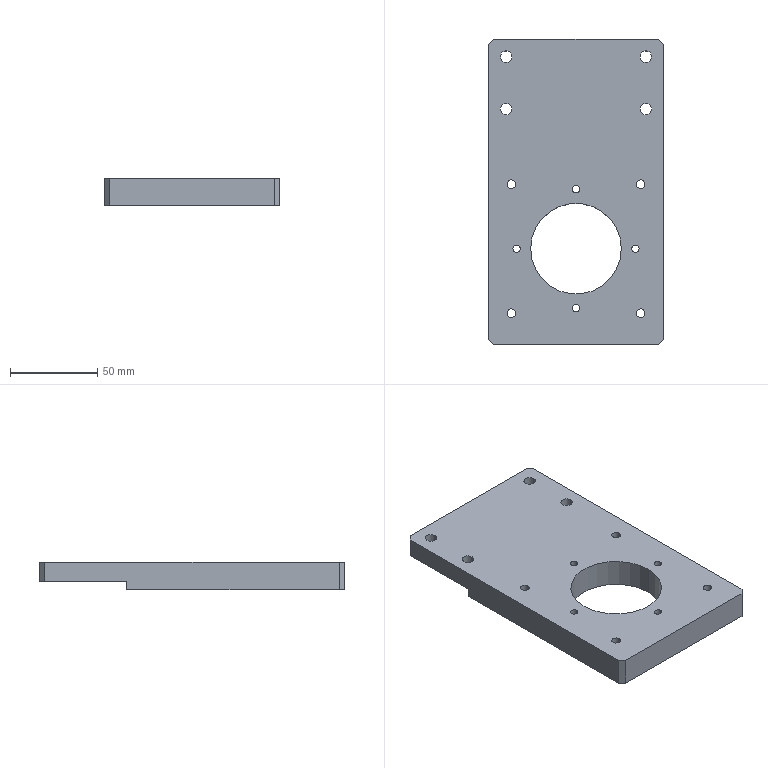Part | STEP file | MT-COMBO-119-S004 | 1 solid | 38 faces | box 100 x 175 x 16 mm | volume 217129 mm3 | cylinder 26 | plane 12 | commonest cylinder face diameters 4.2 x8 5 x8 6.6 x8 52 x2
STEP:
#1=CARTESIAN_POINT('',(36.1,-32.5,0.));
#2=VERTEX_POINT('',#1);
#3=CARTESIAN_POINT('',(31.9,-32.5,0.));
#4=VERTEX_POINT('',#3);
#5=CARTESIAN_POINT('',(34.,-32.5,0.));
#6=DIRECTION('',(0.,0.,-1.));
#7=DIRECTION('',(-1.,0.,0.));
#8=AXIS2_PLACEMENT_3D('',#5,#6,#7);
#9=CIRCLE('',#8,2.1);
#10=EDGE_CURVE('',#2,#4,#9,.T.);
#11=ORIENTED_EDGE('',*,*,#10,.F.);
#12=CARTESIAN_POINT('',(36.1,-32.5,-16.));
#13=VERTEX_POINT('',#12);
#14=CARTESIAN_POINT('',(36.1,-32.5,-16.));
#15=DIRECTION('',(0.,0.,-1.));
#16=VECTOR('',#15,1000.);
#17=LINE('',#14,#16);
#18=EDGE_CURVE('',#2,#13,#17,.T.);
#19=ORIENTED_EDGE('',*,*,#18,.T.);
#20=CARTESIAN_POINT('',(31.9,-32.5,-16.));
#21=VERTEX_POINT('',#20);
#22=CARTESIAN_POINT('',(34.,-32.5,-16.));
#23=DIRECTION('',(0.,0.,-1.));
#24=DIRECTION('',(-1.,0.,0.));
#25=AXIS2_PLACEMENT_3D('',#22,#23,#24);
#26=CIRCLE('',#25,2.1);
#27=EDGE_CURVE('',#13,#21,#26,.T.);
#28=ORIENTED_EDGE('',*,*,#27,.T.);
#29=CARTESIAN_POINT('',(31.9,-32.5,-16.));
#30=DIRECTION('',(0.,0.,-1.));
#31=VECTOR('',#30,1000.);
#32=LINE('',#29,#31);
#33=EDGE_CURVE('',#4,#21,#32,.T.);
#34=ORIENTED_EDGE('',*,*,#33,.F.);
#35=EDGE_LOOP('',(#11,#19,#28,#34));
#36=FACE_OUTER_BOUND('',#35,.T.);
#37=CARTESIAN_POINT('',(34.,-32.5,-16.));
#38=DIRECTION('',(0.,0.,-1.));
#39=DIRECTION('',(-1.,0.,0.));
#40=AXIS2_PLACEMENT_3D('',#37,#38,#39);
#41=CYLINDRICAL_SURFACE('',#40,2.1);
#42=ADVANCED_FACE('',(#36),#41,.F.);
#43=CARTESIAN_POINT('',(2.1,1.5,0.));
#44=VERTEX_POINT('',#43);
#45=CARTESIAN_POINT('',(-2.1,1.5,0.));
#46=VERTEX_POINT('',#45);
#47=CARTESIAN_POINT('',(0.,1.5,0.));
#48=DIRECTION('',(0.,0.,-1.));
#49=DIRECTION('',(-1.,0.,0.));
#50=AXIS2_PLACEMENT_3D('',#47,#48,#49);
#51=CIRCLE('',#50,2.1);
#52=EDGE_CURVE('',#44,#46,#51,.T.);
#53=ORIENTED_EDGE('',*,*,#52,.F.);
#54=CARTESIAN_POINT('',(2.1,1.5,-16.));
#55=VERTEX_POINT('',#54);
#56=CARTESIAN_POINT('',(2.1,1.5,-16.));
#57=DIRECTION('',(0.,0.,-1.));
#58=VECTOR('',#57,1000.);
#59=LINE('',#56,#58);
#60=EDGE_CURVE('',#44,#55,#59,.T.);
#61=ORIENTED_EDGE('',*,*,#60,.T.);
#62=CARTESIAN_POINT('',(-2.1,1.5,-16.));
#63=VERTEX_POINT('',#62);
#64=CARTESIAN_POINT('',(0.,1.5,-16.));
#65=DIRECTION('',(0.,0.,-1.));
#66=DIRECTION('',(-1.,0.,0.));
#67=AXIS2_PLACEMENT_3D('',#64,#65,#66);
#68=CIRCLE('',#67,2.1);
#69=EDGE_CURVE('',#55,#63,#68,.T.);
#70=ORIENTED_EDGE('',*,*,#69,.T.);
#71=CARTESIAN_POINT('',(-2.1,1.5,-16.));
#72=DIRECTION('',(0.,0.,-1.));
#73=VECTOR('',#72,1000.);
#74=LINE('',#71,#73);
#75=EDGE_CURVE('',#46,#63,#74,.T.);
#76=ORIENTED_EDGE('',*,*,#75,.F.);
#77=EDGE_LOOP('',(#53,#61,#70,#76));
#78=FACE_OUTER_BOUND('',#77,.T.);
#79=CARTESIAN_POINT('',(0.,1.5,-16.));
#80=DIRECTION('',(0.,0.,-1.));
#81=DIRECTION('',(-1.,0.,0.));
#82=AXIS2_PLACEMENT_3D('',#79,#80,#81);
#83=CYLINDRICAL_SURFACE('',#82,2.1);
#84=ADVANCED_FACE('',(#78),#83,.F.);
#85=CARTESIAN_POINT('',(2.1,-66.5,0.));
#86=VERTEX_POINT('',#85);
#87=CARTESIAN_POINT('',(-2.1,-66.5,0.));
#88=VERTEX_POINT('',#87);
#89=CARTESIAN_POINT('',(0.,-66.5,0.));
#90=DIRECTION('',(0.,0.,-1.));
#91=DIRECTION('',(-1.,0.,0.));
#92=AXIS2_PLACEMENT_3D('',#89,#90,#91);
#93=CIRCLE('',#92,2.1);
#94=EDGE_CURVE('',#86,#88,#93,.T.);
#95=ORIENTED_EDGE('',*,*,#94,.F.);
#96=CARTESIAN_POINT('',(2.1,-66.5,-16.));
#97=VERTEX_POINT('',#96);
#98=CARTESIAN_POINT('',(2.1,-66.5,-16.));
#99=DIRECTION('',(0.,0.,-1.));
#100=VECTOR('',#99,1000.);
#101=LINE('',#98,#100);
#102=EDGE_CURVE('',#86,#97,#101,.T.);
#103=ORIENTED_EDGE('',*,*,#102,.T.);
#104=CARTESIAN_POINT('',(-2.1,-66.5,-16.));
#105=VERTEX_POINT('',#104);
#106=CARTESIAN_POINT('',(0.,-66.5,-16.));
#107=DIRECTION('',(0.,0.,-1.));
#108=DIRECTION('',(-1.,0.,0.));
#109=AXIS2_PLACEMENT_3D('',#106,#107,#108);
#110=CIRCLE('',#109,2.1);
#111=EDGE_CURVE('',#97,#105,#110,.T.);
#112=ORIENTED_EDGE('',*,*,#111,.T.);
#113=CARTESIAN_POINT('',(-2.1,-66.5,-16.));
#114=DIRECTION('',(0.,0.,-1.));
#115=VECTOR('',#114,1000.);
#116=LINE('',#113,#115);
#117=EDGE_CURVE('',#88,#105,#116,.T.);
#118=ORIENTED_EDGE('',*,*,#117,.F.);
#119=EDGE_LOOP('',(#95,#103,#112,#118));
#120=FACE_OUTER_BOUND('',#119,.T.);
#121=CARTESIAN_POINT('',(0.,-66.5,-16.));
#122=DIRECTION('',(0.,0.,-1.));
#123=DIRECTION('',(-1.,0.,0.));
#124=AXIS2_PLACEMENT_3D('',#121,#122,#123);
#125=CYLINDRICAL_SURFACE('',#124,2.1);
#126=ADVANCED_FACE('',(#120),#125,.F.);
#127=CARTESIAN_POINT('',(-31.9,-32.5,0.));
#128=VERTEX_POINT('',#127);
#129=CARTESIAN_POINT('',(-36.1,-32.5,0.));
#130=VERTEX_POINT('',#129);
#131=CARTESIAN_POINT('',(-34.,-32.5,0.));
#132=DIRECTION('',(0.,0.,-1.));
#133=DIRECTION('',(-1.,0.,0.));
#134=AXIS2_PLACEMENT_3D('',#131,#132,#133);
#135=CIRCLE('',#134,2.1);
#136=EDGE_CURVE('',#128,#130,#135,.T.);
#137=ORIENTED_EDGE('',*,*,#136,.F.);
#138=CARTESIAN_POINT('',(-31.9,-32.5,-16.));
#139=VERTEX_POINT('',#138);
#140=CARTESIAN_POINT('',(-31.9,-32.5,-16.));
#141=DIRECTION('',(0.,0.,-1.));
#142=VECTOR('',#141,1000.);
#143=LINE('',#140,#142);
#144=EDGE_CURVE('',#128,#139,#143,.T.);
#145=ORIENTED_EDGE('',*,*,#144,.T.);
#146=CARTESIAN_POINT('',(-36.1,-32.5,-16.));
#147=VERTEX_POINT('',#146);
#148=CARTESIAN_POINT('',(-34.,-32.5,-16.));
#149=DIRECTION('',(0.,0.,-1.));
#150=DIRECTION('',(-1.,0.,0.));
#151=AXIS2_PLACEMENT_3D('',#148,#149,#150);
#152=CIRCLE('',#151,2.1);
#153=EDGE_CURVE('',#139,#147,#152,.T.);
#154=ORIENTED_EDGE('',*,*,#153,.T.);
#155=CARTESIAN_POINT('',(-36.1,-32.5,-16.));
#156=DIRECTION('',(0.,0.,-1.));
#157=VECTOR('',#156,1000.);
#158=LINE('',#155,#157);
#159=EDGE_CURVE('',#130,#147,#158,.T.);
#160=ORIENTED_EDGE('',*,*,#159,.F.);
#161=EDGE_LOOP('',(#137,#145,#154,#160));
#162=FACE_OUTER_BOUND('',#161,.T.);
#163=CARTESIAN_POINT('',(-34.,-32.5,-16.));
#164=DIRECTION('',(0.,0.,-1.));
#165=DIRECTION('',(-1.,0.,0.));
#166=AXIS2_PLACEMENT_3D('',#163,#164,#165);
#167=CYLINDRICAL_SURFACE('',#166,2.1);
#168=ADVANCED_FACE('',(#162),#167,.F.);
#169=CARTESIAN_POINT('',(-39.5,-69.5,-16.));
#170=VERTEX_POINT('',#169);
#171=CARTESIAN_POINT('',(-34.5,-69.5,-16.));
#172=VERTEX_POINT('',#171);
#173=CARTESIAN_POINT('',(-37.,-69.5,-16.));
#174=DIRECTION('',(0.,0.,-1.));
#175=DIRECTION('',(-1.,0.,0.));
#176=AXIS2_PLACEMENT_3D('',#173,#174,#175);
#177=CIRCLE('',#176,2.5);
#178=EDGE_CURVE('',#170,#172,#177,.T.);
#179=ORIENTED_EDGE('',*,*,#178,.T.);
#180=CARTESIAN_POINT('',(-34.5,-69.5,0.));
#181=VERTEX_POINT('',#180);
#182=CARTESIAN_POINT('',(-34.5,-69.5,0.));
#183=DIRECTION('',(0.,0.,1.));
#184=VECTOR('',#183,1000.);
#185=LINE('',#182,#184);
#186=EDGE_CURVE('',#172,#181,#185,.T.);
#187=ORIENTED_EDGE('',*,*,#186,.T.);
#188=CARTESIAN_POINT('',(-39.5,-69.5,0.));
#189=VERTEX_POINT('',#188);
#190=CARTESIAN_POINT('',(-37.,-69.5,0.));
#191=DIRECTION('',(0.,0.,-1.));
#192=DIRECTION('',(-1.,0.,0.));
#193=AXIS2_PLACEMENT_3D('',#190,#191,#192);
#194=CIRCLE('',#193,2.5);
#195=EDGE_CURVE('',#189,#181,#194,.T.);
#196=ORIENTED_EDGE('',*,*,#195,.F.);
#197=CARTESIAN_POINT('',(-39.5,-69.5,0.));
#198=DIRECTION('',(0.,0.,1.));
#199=VECTOR('',#198,1000.);
#200=LINE('',#197,#199);
#201=EDGE_CURVE('',#170,#189,#200,.T.);
#202=ORIENTED_EDGE('',*,*,#201,.F.);
#203=EDGE_LOOP('',(#179,#187,#196,#202));
#204=FACE_OUTER_BOUND('',#203,.T.);
#205=CARTESIAN_POINT('',(-37.,-69.5,0.));
#206=DIRECTION('',(0.,0.,1.));
#207=DIRECTION('',(-1.,0.,0.));
#208=AXIS2_PLACEMENT_3D('',#205,#206,#207);
#209=CYLINDRICAL_SURFACE('',#208,2.5);
#210=ADVANCED_FACE('',(#204),#209,.F.);
#211=CARTESIAN_POINT('',(34.5,-69.5,-16.));
#212=VERTEX_POINT('',#211);
#213=CARTESIAN_POINT('',(39.5,-69.5,-16.));
#214=VERTEX_POINT('',#213);
#215=CARTESIAN_POINT('',(37.,-69.5,-16.));
#216=DIRECTION('',(0.,0.,-1.));
#217=DIRECTION('',(-1.,0.,0.));
#218=AXIS2_PLACEMENT_3D('',#215,#216,#217);
#219=CIRCLE('',#218,2.5);
#220=EDGE_CURVE('',#212,#214,#219,.T.);
#221=ORIENTED_EDGE('',*,*,#220,.T.);
#222=CARTESIAN_POINT('',(39.5,-69.5,0.));
#223=VERTEX_POINT('',#222);
#224=CARTESIAN_POINT('',(39.5,-69.5,0.));
#225=DIRECTION('',(0.,0.,1.));
#226=VECTOR('',#225,1000.);
#227=LINE('',#224,#226);
#228=EDGE_CURVE('',#214,#223,#227,.T.);
#229=ORIENTED_EDGE('',*,*,#228,.T.);
#230=CARTESIAN_POINT('',(34.5,-69.5,0.));
#231=VERTEX_POINT('',#230);
#232=CARTESIAN_POINT('',(37.,-69.5,0.));
#233=DIRECTION('',(0.,0.,-1.));
#234=DIRECTION('',(-1.,0.,0.));
#235=AXIS2_PLACEMENT_3D('',#232,#233,#234);
#236=CIRCLE('',#235,2.5);
#237=EDGE_CURVE('',#231,#223,#236,.T.);
#238=ORIENTED_EDGE('',*,*,#237,.F.);
#239=CARTESIAN_POINT('',(34.5,-69.5,0.));
#240=DIRECTION('',(0.,0.,1.));
#241=VECTOR('',#240,1000.);
#242=LINE('',#239,#241);
#243=EDGE_CURVE('',#212,#231,#242,.T.);
#244=ORIENTED_EDGE('',*,*,#243,.F.);
#245=EDGE_LOOP('',(#221,#229,#238,#244));
#246=FACE_OUTER_BOUND('',#245,.T.);
#247=CARTESIAN_POINT('',(37.,-69.5,0.));
#248=DIRECTION('',(0.,0.,1.));
#249=DIRECTION('',(-1.,0.,0.));
#250=AXIS2_PLACEMENT_3D('',#247,#248,#249);
#251=CYLINDRICAL_SURFACE('',#250,2.5);
#252=ADVANCED_FACE('',(#246),#251,.F.);
#253=CARTESIAN_POINT('',(34.5,4.5,-16.));
#254=VERTEX_POINT('',#253);
#255=CARTESIAN_POINT('',(39.5,4.5,-16.));
#256=VERTEX_POINT('',#255);
#257=CARTESIAN_POINT('',(37.,4.5,-16.));
#258=DIRECTION('',(0.,0.,-1.));
#259=DIRECTION('',(-1.,0.,0.));
#260=AXIS2_PLACEMENT_3D('',#257,#258,#259);
#261=CIRCLE('',#260,2.5);
#262=EDGE_CURVE('',#254,#256,#261,.T.);
#263=ORIENTED_EDGE('',*,*,#262,.T.);
#264=CARTESIAN_POINT('',(39.5,4.5,0.));
#265=VERTEX_POINT('',#264);
#266=CARTESIAN_POINT('',(39.5,4.5,0.));
#267=DIRECTION('',(0.,0.,1.));
#268=VECTOR('',#267,1000.);
#269=LINE('',#266,#268);
#270=EDGE_CURVE('',#256,#265,#269,.T.);
#271=ORIENTED_EDGE('',*,*,#270,.T.);
#272=CARTESIAN_POINT('',(34.5,4.5,0.));
#273=VERTEX_POINT('',#272);
#274=CARTESIAN_POINT('',(37.,4.5,0.));
#275=DIRECTION('',(0.,0.,-1.));
#276=DIRECTION('',(-1.,0.,0.));
#277=AXIS2_PLACEMENT_3D('',#274,#275,#276);
#278=CIRCLE('',#277,2.5);
#279=EDGE_CURVE('',#273,#265,#278,.T.);
#280=ORIENTED_EDGE('',*,*,#279,.F.);
#281=CARTESIAN_POINT('',(34.5,4.5,0.));
#282=DIRECTION('',(0.,0.,1.));
#283=VECTOR('',#282,1000.);
#284=LINE('',#281,#283);
#285=EDGE_CURVE('',#254,#273,#284,.T.);
#286=ORIENTED_EDGE('',*,*,#285,.F.);
#287=EDGE_LOOP('',(#263,#271,#280,#286));
#288=FACE_OUTER_BOUND('',#287,.T.);
#289=CARTESIAN_POINT('',(37.,4.5,0.));
#290=DIRECTION('',(0.,0.,1.));
#291=DIRECTION('',(-1.,0.,0.));
#292=AXIS2_PLACEMENT_3D('',#289,#290,#291);
#293=CYLINDRICAL_SURFACE('',#292,2.5);
#294=ADVANCED_FACE('',(#288),#293,.F.);
#295=CARTESIAN_POINT('',(-39.5,4.5,-16.));
#296=VERTEX_POINT('',#295);
#297=CARTESIAN_POINT('',(-34.5,4.5,-16.));
#298=VERTEX_POINT('',#297);
#299=CARTESIAN_POINT('',(-37.,4.5,-16.));
#300=DIRECTION('',(0.,0.,-1.));
#301=DIRECTION('',(-1.,0.,0.));
#302=AXIS2_PLACEMENT_3D('',#299,#300,#301);
#303=CIRCLE('',#302,2.5);
#304=EDGE_CURVE('',#296,#298,#303,.T.);
#305=ORIENTED_EDGE('',*,*,#304,.T.);
#306=CARTESIAN_POINT('',(-34.5,4.5,0.));
#307=VERTEX_POINT('',#306);
#308=CARTESIAN_POINT('',(-34.5,4.5,0.));
#309=DIRECTION('',(0.,0.,1.));
#310=VECTOR('',#309,1000.);
#311=LINE('',#308,#310);
#312=EDGE_CURVE('',#298,#307,#311,.T.);
#313=ORIENTED_EDGE('',*,*,#312,.T.);
#314=CARTESIAN_POINT('',(-39.5,4.5,0.));
#315=VERTEX_POINT('',#314);
#316=CARTESIAN_POINT('',(-37.,4.5,0.));
#317=DIRECTION('',(0.,0.,-1.));
#318=DIRECTION('',(-1.,0.,0.));
#319=AXIS2_PLACEMENT_3D('',#316,#317,#318);
#320=CIRCLE('',#319,2.5);
#321=EDGE_CURVE('',#315,#307,#320,.T.);
#322=ORIENTED_EDGE('',*,*,#321,.F.);
#323=CARTESIAN_POINT('',(-39.5,4.5,0.));
#324=DIRECTION('',(0.,0.,1.));
#325=VECTOR('',#324,1000.);
#326=LINE('',#323,#325);
#327=EDGE_CURVE('',#296,#315,#326,.T.);
#328=ORIENTED_EDGE('',*,*,#327,.F.);
#329=EDGE_LOOP('',(#305,#313,#322,#328));
#330=FACE_OUTER_BOUND('',#329,.T.);
#331=CARTESIAN_POINT('',(-37.,4.5,0.));
#332=DIRECTION('',(0.,0.,1.));
#333=DIRECTION('',(-1.,0.,0.));
#334=AXIS2_PLACEMENT_3D('',#331,#332,#333);
#335=CYLINDRICAL_SURFACE('',#334,2.5);
#336=ADVANCED_FACE('',(#330),#335,.F.);
#337=CARTESIAN_POINT('',(-43.3,47.5,-11.));
#338=VERTEX_POINT('',#337);
#339=CARTESIAN_POINT('',(-36.7,47.5,-11.));
#340=VERTEX_POINT('',#339);
#341=CARTESIAN_POINT('',(-40.,47.5,-11.));
#342=DIRECTION('',(0.,0.,-1.));
#343=DIRECTION('',(-1.,0.,0.));
#344=AXIS2_PLACEMENT_3D('',#341,#342,#343);
#345=CIRCLE('',#344,3.3);
#346=EDGE_CURVE('',#338,#340,#345,.T.);
#347=ORIENTED_EDGE('',*,*,#346,.T.);
#348=CARTESIAN_POINT('',(-36.7,47.5,0.));
#349=VERTEX_POINT('',#348);
#350=CARTESIAN_POINT('',(-36.7,47.5,0.));
#351=DIRECTION('',(0.,0.,1.));
#352=VECTOR('',#351,1000.);
#353=LINE('',#350,#352);
#354=EDGE_CURVE('',#340,#349,#353,.T.);
#355=ORIENTED_EDGE('',*,*,#354,.T.);
#356=CARTESIAN_POINT('',(-43.3,47.5,0.));
#357=VERTEX_POINT('',#356);
#358=CARTESIAN_POINT('',(-40.,47.5,0.));
#359=DIRECTION('',(0.,0.,-1.));
#360=DIRECTION('',(-1.,0.,0.));
#361=AXIS2_PLACEMENT_3D('',#358,#359,#360);
#362=CIRCLE('',#361,3.3);
#363=EDGE_CURVE('',#357,#349,#362,.T.);
#364=ORIENTED_EDGE('',*,*,#363,.F.);
#365=CARTESIAN_POINT('',(-43.3,47.5,0.));
#366=DIRECTION('',(0.,0.,1.));
#367=VECTOR('',#366,1000.);
#368=LINE('',#365,#367);
#369=EDGE_CURVE('',#338,#357,#368,.T.);
#370=ORIENTED_EDGE('',*,*,#369,.F.);
#371=EDGE_LOOP('',(#347,#355,#364,#370));
#372=FACE_OUTER_BOUND('',#371,.T.);
#373=CARTESIAN_POINT('',(-40.,47.5,0.));
#374=DIRECTION('',(0.,0.,1.));
#375=DIRECTION('',(-1.,0.,0.));
#376=AXIS2_PLACEMENT_3D('',#373,#374,#375);
#377=CYLINDRICAL_SURFACE('',#376,3.3);
#378=ADVANCED_FACE('',(#372),#377,.F.);
#379=CARTESIAN_POINT('',(-43.3,77.5,-11.));
#380=VERTEX_POINT('',#379);
#381=CARTESIAN_POINT('',(-36.7,77.5,-11.));
#382=VERTEX_POINT('',#381);
#383=CARTESIAN_POINT('',(-40.,77.5,-11.));
#384=DIRECTION('',(0.,0.,-1.));
#385=DIRECTION('',(-1.,0.,0.));
#386=AXIS2_PLACEMENT_3D('',#383,#384,#385);
#387=CIRCLE('',#386,3.3);
#388=EDGE_CURVE('',#380,#382,#387,.T.);
#389=ORIENTED_EDGE('',*,*,#388,.T.);
#390=CARTESIAN_POINT('',(-36.7,77.5,0.));
#391=VERTEX_POINT('',#390);
#392=CARTESIAN_POINT('',(-36.7,77.5,0.));
#393=DIRECTION('',(0.,0.,1.));
#394=VECTOR('',#393,1000.);
#395=LINE('',#392,#394);
#396=EDGE_CURVE('',#382,#391,#395,.T.);
#397=ORIENTED_EDGE('',*,*,#396,.T.);
#398=CARTESIAN_POINT('',(-43.3,77.5,0.));
#399=VERTEX_POINT('',#398);
#400=CARTESIAN_POINT('',(-40.,77.5,0.));
#401=DIRECTION('',(0.,0.,-1.));
#402=DIRECTION('',(-1.,0.,0.));
#403=AXIS2_PLACEMENT_3D('',#400,#401,#402);
#404=CIRCLE('',#403,3.3);
#405=EDGE_CURVE('',#399,#391,#404,.T.);
#406=ORIENTED_EDGE('',*,*,#405,.F.);
#407=CARTESIAN_POINT('',(-43.3,77.5,0.));
#408=DIRECTION('',(0.,0.,1.));
#409=VECTOR('',#408,1000.);
#410=LINE('',#407,#409);
#411=EDGE_CURVE('',#380,#399,#410,.T.);
#412=ORIENTED_EDGE('',*,*,#411,.F.);
#413=EDGE_LOOP('',(#389,#397,#406,#412));
#414=FACE_OUTER_BOUND('',#413,.T.);
#415=CARTESIAN_POINT('',(-40.,77.5,0.));
#416=DIRECTION('',(0.,0.,1.));
#417=DIRECTION('',(-1.,0.,0.));
#418=AXIS2_PLACEMENT_3D('',#415,#416,#417);
#419=CYLINDRICAL_SURFACE('',#418,3.3);
#420=ADVANCED_FACE('',(#414),#419,.F.);
#421=CARTESIAN_POINT('',(36.7,77.5,-11.));
#422=VERTEX_POINT('',#421);
#423=CARTESIAN_POINT('',(43.3,77.5,-11.));
#424=VERTEX_POINT('',#423);
#425=CARTESIAN_POINT('',(40.,77.5,-11.));
#426=DIRECTION('',(0.,0.,-1.));
#427=DIRECTION('',(-1.,0.,0.));
#428=AXIS2_PLACEMENT_3D('',#425,#426,#427);
#429=CIRCLE('',#428,3.3);
#430=EDGE_CURVE('',#422,#424,#429,.T.);
#431=ORIENTED_EDGE('',*,*,#430,.T.);
#432=CARTESIAN_POINT('',(43.3,77.5,0.));
#433=VERTEX_POINT('',#432);
#434=CARTESIAN_POINT('',(43.3,77.5,0.));
#435=DIRECTION('',(0.,0.,1.));
#436=VECTOR('',#435,1000.);
#437=LINE('',#434,#436);
#438=EDGE_CURVE('',#424,#433,#437,.T.);
#439=ORIENTED_EDGE('',*,*,#438,.T.);
#440=CARTESIAN_POINT('',(36.7,77.5,0.));
#441=VERTEX_POINT('',#440);
#442=CARTESIAN_POINT('',(40.,77.5,0.));
#443=DIRECTION('',(0.,0.,-1.));
#444=DIRECTION('',(-1.,0.,0.));
#445=AXIS2_PLACEMENT_3D('',#442,#443,#444);
#446=CIRCLE('',#445,3.3);
#447=EDGE_CURVE('',#441,#433,#446,.T.);
#448=ORIENTED_EDGE('',*,*,#447,.F.);
#449=CARTESIAN_POINT('',(36.7,77.5,0.));
#450=DIRECTION('',(0.,0.,1.));
#451=VECTOR('',#450,1000.);
#452=LINE('',#449,#451);
#453=EDGE_CURVE('',#422,#441,#452,.T.);
#454=ORIENTED_EDGE('',*,*,#453,.F.);
#455=EDGE_LOOP('',(#431,#439,#448,#454));
#456=FACE_OUTER_BOUND('',#455,.T.);
#457=CARTESIAN_POINT('',(40.,77.5,0.));
#458=DIRECTION('',(0.,0.,1.));
#459=DIRECTION('',(-1.,0.,0.));
#460=AXIS2_PLACEMENT_3D('',#457,#458,#459);
#461=CYLINDRICAL_SURFACE('',#460,3.3);
#462=ADVANCED_FACE('',(#456),#461,.F.);
#463=CARTESIAN_POINT('',(36.7,47.5,-11.));
#464=VERTEX_POINT('',#463);
#465=CARTESIAN_POINT('',(43.3,47.5,-11.));
#466=VERTEX_POINT('',#465);
#467=CARTESIAN_POINT('',(40.,47.5,-11.));
#468=DIRECTION('',(0.,0.,-1.));
#469=DIRECTION('',(-1.,0.,0.));
#470=AXIS2_PLACEMENT_3D('',#467,#468,#469);
#471=CIRCLE('',#470,3.3);
#472=EDGE_CURVE('',#464,#466,#471,.T.);
#473=ORIENTED_EDGE('',*,*,#472,.T.);
#474=CARTESIAN_POINT('',(43.3,47.5,0.));
#475=VERTEX_POINT('',#474);
#476=CARTESIAN_POINT('',(43.3,47.5,0.));
#477=DIRECTION('',(0.,0.,1.));
#478=VECTOR('',#477,1000.);
#479=LINE('',#476,#478);
#480=EDGE_CURVE('',#466,#475,#479,.T.);
#481=ORIENTED_EDGE('',*,*,#480,.T.);
#482=CARTESIAN_POINT('',(36.7,47.5,0.));
#483=VERTEX_POINT('',#482);
#484=CARTESIAN_POINT('',(40.,47.5,0.));
#485=DIRECTION('',(0.,0.,-1.));
#486=DIRECTION('',(-1.,0.,0.));
#487=AXIS2_PLACEMENT_3D('',#484,#485,#486);
#488=CIRCLE('',#487,3.3);
#489=EDGE_CURVE('',#483,#475,#488,.T.);
#490=ORIENTED_EDGE('',*,*,#489,.F.);
#491=CARTESIAN_POINT('',(36.7,47.5,0.));
#492=DIRECTION('',(0.,0.,1.));
#493=VECTOR('',#492,1000.);
#494=LINE('',#491,#493);
#495=EDGE_CURVE('',#464,#483,#494,.T.);
#496=ORIENTED_EDGE('',*,*,#495,.F.);
#497=EDGE_LOOP('',(#473,#481,#490,#496));
#498=FACE_OUTER_BOUND('',#497,.T.);
#499=CARTESIAN_POINT('',(40.,47.5,0.));
#500=DIRECTION('',(0.,0.,1.));
#501=DIRECTION('',(-1.,0.,0.));
#502=AXIS2_PLACEMENT_3D('',#499,#500,#501);
#503=CYLINDRICAL_SURFACE('',#502,3.3);
#504=ADVANCED_FACE('',(#498),#503,.F.);
#505=CARTESIAN_POINT('',(-26.,-32.5,-16.));
#506=VERTEX_POINT('',#505);
#507=CARTESIAN_POINT('',(26.,-32.5,-16.));
#508=VERTEX_POINT('',#507);
#509=CARTESIAN_POINT('',(0.,-32.5,-16.));
#510=DIRECTION('',(0.,0.,-1.));
#511=DIRECTION('',(-1.,0.,0.));
#512=AXIS2_PLACEMENT_3D('',#509,#510,#511);
#513=CIRCLE('',#512,26.);
#514=EDGE_CURVE('',#506,#508,#513,.T.);
#515=ORIENTED_EDGE('',*,*,#514,.T.);
#516=CARTESIAN_POINT('',(26.,-32.5,0.));
#517=VERTEX_POINT('',#516);
#518=CARTESIAN_POINT('',(26.,-32.5,-16.));
#519=DIRECTION('',(0.,0.,1.));
#520=VECTOR('',#519,1000.);
#521=LINE('',#518,#520);
#522=EDGE_CURVE('',#508,#517,#521,.T.);
#523=ORIENTED_EDGE('',*,*,#522,.T.);
#524=CARTESIAN_POINT('',(-26.,-32.5,0.));
#525=VERTEX_POINT('',#524);
#526=CARTESIAN_POINT('',(0.,-32.5,0.));
#527=DIRECTION('',(0.,0.,-1.));
#528=DIRECTION('',(-1.,0.,0.));
#529=AXIS2_PLACEMENT_3D('',#526,#527,#528);
#530=CIRCLE('',#529,26.);
#531=EDGE_CURVE('',#525,#517,#530,.T.);
#532=ORIENTED_EDGE('',*,*,#531,.F.);
#533=CARTESIAN_POINT('',(-26.,-32.5,-16.));
#534=DIRECTION('',(0.,0.,1.));
#535=VECTOR('',#534,1000.);
#536=LINE('',#533,#535);
#537=EDGE_CURVE('',#506,#525,#536,.T.);
#538=ORIENTED_EDGE('',*,*,#537,.F.);
#539=EDGE_LOOP('',(#515,#523,#532,#538));
#540=FACE_OUTER_BOUND('',#539,.T.);
#541=CARTESIAN_POINT('',(0.,-32.5,-16.));
#542=DIRECTION('',(0.,0.,1.));
#543=DIRECTION('',(-1.,0.,0.));
#544=AXIS2_PLACEMENT_3D('',#541,#542,#543);
#545=CYLINDRICAL_SURFACE('',#544,26.);
#546=ADVANCED_FACE('',(#540),#545,.F.);
#547=CARTESIAN_POINT('',(50.,-84.5,-16.));
#548=VERTEX_POINT('',#547);
#549=CARTESIAN_POINT('',(50.,37.5,-16.));
#550=VERTEX_POINT('',#549);
#551=CARTESIAN_POINT('',(50.,-87.5,-16.));
#552=DIRECTION('',(0.,1.,0.));
#553=VECTOR('',#552,1000.);
#554=LINE('',#551,#553);
#555=EDGE_CURVE('',#548,#550,#554,.T.);
#556=ORIENTED_EDGE('',*,*,#555,.T.);
#557=CARTESIAN_POINT('',(50.,37.5,-11.));
#558=VERTEX_POINT('',#557);
#559=CARTESIAN_POINT('',(50.,37.5,-11.));
#560=DIRECTION('',(0.,0.,-1.));
#561=VECTOR('',#560,1000.);
#562=LINE('',#559,#561);
#563=EDGE_CURVE('',#558,#550,#562,.T.);
#564=ORIENTED_EDGE('',*,*,#563,.F.);
#565=CARTESIAN_POINT('',(50.,84.5,-11.));
#566=VERTEX_POINT('',#565);
#567=CARTESIAN_POINT('',(50.,87.5,-11.));
#568=DIRECTION('',(0.,1.,0.));
#569=VECTOR('',#568,1000.);
#570=LINE('',#567,#569);
#571=EDGE_CURVE('',#558,#566,#570,.T.);
#572=ORIENTED_EDGE('',*,*,#571,.T.);
#573=CARTESIAN_POINT('',(50.,84.5,0.));
#574=VERTEX_POINT('',#573);
#575=CARTESIAN_POINT('',(50.,84.5,-16.));
#576=DIRECTION('',(0.,0.,-1.));
#577=VECTOR('',#576,1000.);
#578=LINE('',#575,#577);
#579=EDGE_CURVE('',#574,#566,#578,.T.);
#580=ORIENTED_EDGE('',*,*,#579,.F.);
#581=CARTESIAN_POINT('',(50.,-84.5,0.));
#582=VERTEX_POINT('',#581);
#583=CARTESIAN_POINT('',(50.,-87.5,0.));
#584=DIRECTION('',(0.,1.,0.));
#585=VECTOR('',#584,1000.);
#586=LINE('',#583,#585);
#587=EDGE_CURVE('',#582,#574,#586,.T.);
#588=ORIENTED_EDGE('',*,*,#587,.F.);
#589=CARTESIAN_POINT('',(50.,-84.5,-16.));
#590=DIRECTION('',(0.,0.,1.));
#591=VECTOR('',#590,1000.);
#592=LINE('',#589,#591);
#593=EDGE_CURVE('',#548,#582,#592,.T.);
#594=ORIENTED_EDGE('',*,*,#593,.F.);
#595=EDGE_LOOP('',(#556,#564,#572,#580,#588,#594));
#596=FACE_OUTER_BOUND('',#595,.T.);
#597=CARTESIAN_POINT('',(50.,-87.5,-16.));
#598=DIRECTION('',(-1.,0.,0.));
#599=DIRECTION('',(0.,0.,-1.));
#600=AXIS2_PLACEMENT_3D('',#597,#598,#599);
#601=PLANE('',#600);
#602=ADVANCED_FACE('',(#596),#601,.F.);
#603=CARTESIAN_POINT('',(47.,87.5,0.));
#604=VERTEX_POINT('',#603);
#605=CARTESIAN_POINT('',(-47.,87.5,0.));
#606=VERTEX_POINT('',#605);
#607=CARTESIAN_POINT('',(-50.,87.5,0.));
#608=DIRECTION('',(-1.,0.,0.));
#609=VECTOR('',#608,1000.);
#610=LINE('',#607,#609);
#611=EDGE_CURVE('',#604,#606,#610,.T.);
#612=ORIENTED_EDGE('',*,*,#611,.F.);
#613=CARTESIAN_POINT('',(47.,87.5,-11.));
#614=VERTEX_POINT('',#613);
#615=CARTESIAN_POINT('',(47.,87.5,-16.));
#616=DIRECTION('',(0.,0.,1.));
#617=VECTOR('',#616,1000.);
#618=LINE('',#615,#617);
#619=EDGE_CURVE('',#614,#604,#618,.T.);
#620=ORIENTED_EDGE('',*,*,#619,.F.);
#621=CARTESIAN_POINT('',(-47.,87.5,-11.));
#622=VERTEX_POINT('',#621);
#623=CARTESIAN_POINT('',(50.,87.5,-11.));
#624=DIRECTION('',(-1.,0.,0.));
#625=VECTOR('',#624,1000.);
#626=LINE('',#623,#625);
#627=EDGE_CURVE('',#614,#622,#626,.T.);
#628=ORIENTED_EDGE('',*,*,#627,.T.);
#629=CARTESIAN_POINT('',(-47.,87.5,-16.));
#630=DIRECTION('',(0.,0.,-1.));
#631=VECTOR('',#630,1000.);
#632=LINE('',#629,#631);
#633=EDGE_CURVE('',#606,#622,#632,.T.);
#634=ORIENTED_EDGE('',*,*,#633,.F.);
#635=EDGE_LOOP('',(#612,#620,#628,#634));
#636=FACE_OUTER_BOUND('',#635,.T.);
#637=CARTESIAN_POINT('',(-50.,87.5,-16.));
#638=DIRECTION('',(0.,-1.,0.));
#639=DIRECTION('',(0.,0.,1.));
#640=AXIS2_PLACEMENT_3D('',#637,#638,#639);
#641=PLANE('',#640);
#642=ADVANCED_FACE('',(#636),#641,.F.);
#643=CARTESIAN_POINT('',(-50.,84.5,0.));
#644=VERTEX_POINT('',#643);
#645=CARTESIAN_POINT('',(-50.,-84.5,0.));
#646=VERTEX_POINT('',#645);
#647=CARTESIAN_POINT('',(-50.,-87.5,0.));
#648=DIRECTION('',(0.,-1.,0.));
#649=VECTOR('',#648,1000.);
#650=LINE('',#647,#649);
#651=EDGE_CURVE('',#644,#646,#650,.T.);
#652=ORIENTED_EDGE('',*,*,#651,.F.);
#653=CARTESIAN_POINT('',(-50.,84.5,-11.));
#654=VERTEX_POINT('',#653);
#655=CARTESIAN_POINT('',(-50.,84.5,-16.));
#656=DIRECTION('',(0.,0.,1.));
#657=VECTOR('',#656,1000.);
#658=LINE('',#655,#657);
#659=EDGE_CURVE('',#654,#644,#658,.T.);
#660=ORIENTED_EDGE('',*,*,#659,.F.);
#661=CARTESIAN_POINT('',(-50.,37.5,-11.));
#662=VERTEX_POINT('',#661);
#663=CARTESIAN_POINT('',(-50.,87.5,-11.));
#664=DIRECTION('',(0.,-1.,0.));
#665=VECTOR('',#664,1000.);
#666=LINE('',#663,#665);
#667=EDGE_CURVE('',#654,#662,#666,.T.);
#668=ORIENTED_EDGE('',*,*,#667,.T.);
#669=CARTESIAN_POINT('',(-50.,37.5,-16.));
#670=VERTEX_POINT('',#669);
#671=CARTESIAN_POINT('',(-50.,37.5,-11.));
#672=DIRECTION('',(0.,0.,-1.));
#673=VECTOR('',#672,1000.);
#674=LINE('',#671,#673);
#675=EDGE_CURVE('',#662,#670,#674,.T.);
#676=ORIENTED_EDGE('',*,*,#675,.T.);
#677=CARTESIAN_POINT('',(-50.,-84.5,-16.));
#678=VERTEX_POINT('',#677);
#679=CARTESIAN_POINT('',(-50.,-87.5,-16.));
#680=DIRECTION('',(0.,-1.,0.));
#681=VECTOR('',#680,1000.);
#682=LINE('',#679,#681);
#683=EDGE_CURVE('',#670,#678,#682,.T.);
#684=ORIENTED_EDGE('',*,*,#683,.T.);
#685=CARTESIAN_POINT('',(-50.,-84.5,-16.));
#686=DIRECTION('',(0.,0.,-1.));
#687=VECTOR('',#686,1000.);
#688=LINE('',#685,#687);
#689=EDGE_CURVE('',#646,#678,#688,.T.);
#690=ORIENTED_EDGE('',*,*,#689,.F.);
#691=EDGE_LOOP('',(#652,#660,#668,#676,#684,#690));
#692=FACE_OUTER_BOUND('',#691,.T.);
#693=CARTESIAN_POINT('',(-50.,-87.5,-16.));
#694=DIRECTION('',(1.,0.,0.));
#695=DIRECTION('',(0.,0.,1.));
#696=AXIS2_PLACEMENT_3D('',#693,#694,#695);
#697=PLANE('',#696);
#698=ADVANCED_FACE('',(#692),#697,.F.);
#699=CARTESIAN_POINT('',(-47.,-87.5,-16.));
#700=VERTEX_POINT('',#699);
#701=CARTESIAN_POINT('',(47.,-87.5,-16.));
#702=VERTEX_POINT('',#701);
#703=CARTESIAN_POINT('',(-50.,-87.5,-16.));
#704=DIRECTION('',(1.,0.,0.));
#705=VECTOR('',#704,1000.);
#706=LINE('',#703,#705);
#707=EDGE_CURVE('',#700,#702,#706,.T.);
#708=ORIENTED_EDGE('',*,*,#707,.T.);
#709=CARTESIAN_POINT('',(47.,-87.5,0.));
#710=VERTEX_POINT('',#709);
#711=CARTESIAN_POINT('',(47.,-87.5,-16.));
#712=DIRECTION('',(0.,0.,-1.));
#713=VECTOR('',#712,1000.);
#714=LINE('',#711,#713);
#715=EDGE_CURVE('',#710,#702,#714,.T.);
#716=ORIENTED_EDGE('',*,*,#715,.F.);
#717=CARTESIAN_POINT('',(-47.,-87.5,0.));
#718=VERTEX_POINT('',#717);
#719=CARTESIAN_POINT('',(-50.,-87.5,0.));
#720=DIRECTION('',(1.,0.,0.));
#721=VECTOR('',#720,1000.);
#722=LINE('',#719,#721);
#723=EDGE_CURVE('',#718,#710,#722,.T.);
#724=ORIENTED_EDGE('',*,*,#723,.F.);
#725=CARTESIAN_POINT('',(-47.,-87.5,-16.));
#726=DIRECTION('',(0.,0.,1.));
#727=VECTOR('',#726,1000.);
#728=LINE('',#725,#727);
#729=EDGE_CURVE('',#700,#718,#728,.T.);
#730=ORIENTED_EDGE('',*,*,#729,.F.);
#731=EDGE_LOOP('',(#708,#716,#724,#730));
#732=FACE_OUTER_BOUND('',#731,.T.);
#733=CARTESIAN_POINT('',(-50.,-87.5,-16.));
#734=DIRECTION('',(0.,1.,0.));
#735=DIRECTION('',(0.,0.,-1.));
#736=AXIS2_PLACEMENT_3D('',#733,#734,#735);
#737=PLANE('',#736);
#738=ADVANCED_FACE('',(#732),#737,.F.);
#739=CARTESIAN_POINT('',(34.,-32.5,-16.));
#740=DIRECTION('',(0.,0.,-1.));
#741=DIRECTION('',(-1.,0.,0.));
#742=AXIS2_PLACEMENT_3D('',#739,#740,#741);
#743=CIRCLE('',#742,2.1);
#744=EDGE_CURVE('',#21,#13,#743,.T.);
#745=ORIENTED_EDGE('',*,*,#744,.F.);
#746=ORIENTED_EDGE('',*,*,#27,.F.);
#747=EDGE_LOOP('',(#745,#746));
#748=FACE_BOUND('',#747,.T.);
#749=CARTESIAN_POINT('',(0.,1.5,-16.));
#750=DIRECTION('',(0.,0.,-1.));
#751=DIRECTION('',(-1.,0.,0.));
#752=AXIS2_PLACEMENT_3D('',#749,#750,#751);
#753=CIRCLE('',#752,2.1);
#754=EDGE_CURVE('',#63,#55,#753,.T.);
#755=ORIENTED_EDGE('',*,*,#754,.F.);
#756=ORIENTED_EDGE('',*,*,#69,.F.);
#757=EDGE_LOOP('',(#755,#756));
#758=FACE_BOUND('',#757,.T.);
#759=CARTESIAN_POINT('',(0.,-66.5,-16.));
#760=DIRECTION('',(0.,0.,-1.));
#761=DIRECTION('',(-1.,0.,0.));
#762=AXIS2_PLACEMENT_3D('',#759,#760,#761);
#763=CIRCLE('',#762,2.1);
#764=EDGE_CURVE('',#105,#97,#763,.T.);
#765=ORIENTED_EDGE('',*,*,#764,.F.);
#766=ORIENTED_EDGE('',*,*,#111,.F.);
#767=EDGE_LOOP('',(#765,#766));
#768=FACE_BOUND('',#767,.T.);
#769=CARTESIAN_POINT('',(-34.,-32.5,-16.));
#770=DIRECTION('',(0.,0.,-1.));
#771=DIRECTION('',(-1.,0.,0.));
#772=AXIS2_PLACEMENT_3D('',#769,#770,#771);
#773=CIRCLE('',#772,2.1);
#774=EDGE_CURVE('',#147,#139,#773,.T.);
#775=ORIENTED_EDGE('',*,*,#774,.F.);
#776=ORIENTED_EDGE('',*,*,#153,.F.);
#777=EDGE_LOOP('',(#775,#776));
#778=FACE_BOUND('',#777,.T.);
#779=ORIENTED_EDGE('',*,*,#178,.F.);
#780=CARTESIAN_POINT('',(-37.,-69.5,-16.));
#781=DIRECTION('',(0.,0.,-1.));
#782=DIRECTION('',(-1.,0.,0.));
#783=AXIS2_PLACEMENT_3D('',#780,#781,#782);
#784=CIRCLE('',#783,2.5);
#785=EDGE_CURVE('',#172,#170,#784,.T.);
#786=ORIENTED_EDGE('',*,*,#785,.F.);
#787=EDGE_LOOP('',(#779,#786));
#788=FACE_BOUND('',#787,.T.);
#789=ORIENTED_EDGE('',*,*,#220,.F.);
#790=CARTESIAN_POINT('',(37.,-69.5,-16.));
#791=DIRECTION('',(0.,0.,-1.));
#792=DIRECTION('',(-1.,0.,0.));
#793=AXIS2_PLACEMENT_3D('',#790,#791,#792);
#794=CIRCLE('',#793,2.5);
#795=EDGE_CURVE('',#214,#212,#794,.T.);
#796=ORIENTED_EDGE('',*,*,#795,.F.);
#797=EDGE_LOOP('',(#789,#796));
#798=FACE_BOUND('',#797,.T.);
#799=ORIENTED_EDGE('',*,*,#262,.F.);
#800=CARTESIAN_POINT('',(37.,4.5,-16.));
#801=DIRECTION('',(0.,0.,-1.));
#802=DIRECTION('',(-1.,0.,0.));
#803=AXIS2_PLACEMENT_3D('',#800,#801,#802);
#804=CIRCLE('',#803,2.5);
#805=EDGE_CURVE('',#256,#254,#804,.T.);
#806=ORIENTED_EDGE('',*,*,#805,.F.);
#807=EDGE_LOOP('',(#799,#806));
#808=FACE_BOUND('',#807,.T.);
#809=ORIENTED_EDGE('',*,*,#304,.F.);
#810=CARTESIAN_POINT('',(-37.,4.5,-16.));
#811=DIRECTION('',(0.,0.,-1.));
#812=DIRECTION('',(-1.,0.,0.));
#813=AXIS2_PLACEMENT_3D('',#810,#811,#812);
#814=CIRCLE('',#813,2.5);
#815=EDGE_CURVE('',#298,#296,#814,.T.);
#816=ORIENTED_EDGE('',*,*,#815,.F.);
#817=EDGE_LOOP('',(#809,#816));
#818=FACE_BOUND('',#817,.T.);
#819=ORIENTED_EDGE('',*,*,#514,.F.);
#820=CARTESIAN_POINT('',(0.,-32.5,-16.));
#821=DIRECTION('',(0.,0.,-1.));
#822=DIRECTION('',(-1.,0.,0.));
#823=AXIS2_PLACEMENT_3D('',#820,#821,#822);
#824=CIRCLE('',#823,26.);
#825=EDGE_CURVE('',#508,#506,#824,.T.);
#826=ORIENTED_EDGE('',*,*,#825,.F.);
#827=EDGE_LOOP('',(#819,#826));
#828=FACE_BOUND('',#827,.T.);
#829=ORIENTED_EDGE('',*,*,#683,.F.);
#830=CARTESIAN_POINT('',(50.,37.5,-16.));
#831=DIRECTION('',(1.,0.,0.));
#832=VECTOR('',#831,1000.);
#833=LINE('',#830,#832);
#834=EDGE_CURVE('',#670,#550,#833,.T.);
#835=ORIENTED_EDGE('',*,*,#834,.T.);
#836=ORIENTED_EDGE('',*,*,#555,.F.);
#837=CARTESIAN_POINT('',(50.,-84.5,-16.));
#838=DIRECTION('',(0.7071,0.7071,0.));
#839=VECTOR('',#838,1000.);
#840=LINE('',#837,#839);
#841=EDGE_CURVE('',#702,#548,#840,.T.);
#842=ORIENTED_EDGE('',*,*,#841,.F.);
#843=ORIENTED_EDGE('',*,*,#707,.F.);
#844=CARTESIAN_POINT('',(-47.,-87.5,-16.));
#845=DIRECTION('',(0.7071,-0.7071,0.));
#846=VECTOR('',#845,1000.);
#847=LINE('',#844,#846);
#848=EDGE_CURVE('',#678,#700,#847,.T.);
#849=ORIENTED_EDGE('',*,*,#848,.F.);
#850=EDGE_LOOP('',(#829,#835,#836,#842,#843,#849));
#851=FACE_OUTER_BOUND('',#850,.T.);
#852=CARTESIAN_POINT('',(0.,0.,-16.));
#853=DIRECTION('',(0.,0.,1.));
#854=DIRECTION('',(-1.,0.,0.));
#855=AXIS2_PLACEMENT_3D('',#852,#853,#854);
#856=PLANE('',#855);
#857=ADVANCED_FACE('',(#748,#758,#768,#778,#788,#798,#808,#818,#828,#851),#856,.F.);
#858=CARTESIAN_POINT('',(34.,-32.5,0.));
#859=DIRECTION('',(0.,0.,-1.));
#860=DIRECTION('',(-1.,0.,0.));
#861=AXIS2_PLACEMENT_3D('',#858,#859,#860);
#862=CIRCLE('',#861,2.1);
#863=EDGE_CURVE('',#4,#2,#862,.T.);
#864=ORIENTED_EDGE('',*,*,#863,.T.);
#865=ORIENTED_EDGE('',*,*,#10,.T.);
#866=EDGE_LOOP('',(#864,#865));
#867=FACE_BOUND('',#866,.T.);
#868=CARTESIAN_POINT('',(0.,1.5,0.));
#869=DIRECTION('',(0.,0.,-1.));
#870=DIRECTION('',(-1.,0.,0.));
#871=AXIS2_PLACEMENT_3D('',#868,#869,#870);
#872=CIRCLE('',#871,2.1);
#873=EDGE_CURVE('',#46,#44,#872,.T.);
#874=ORIENTED_EDGE('',*,*,#873,.T.);
#875=ORIENTED_EDGE('',*,*,#52,.T.);
#876=EDGE_LOOP('',(#874,#875));
#877=FACE_BOUND('',#876,.T.);
#878=CARTESIAN_POINT('',(0.,-66.5,0.));
#879=DIRECTION('',(0.,0.,-1.));
#880=DIRECTION('',(-1.,0.,0.));
#881=AXIS2_PLACEMENT_3D('',#878,#879,#880);
#882=CIRCLE('',#881,2.1);
#883=EDGE_CURVE('',#88,#86,#882,.T.);
#884=ORIENTED_EDGE('',*,*,#883,.T.);
#885=ORIENTED_EDGE('',*,*,#94,.T.);
#886=EDGE_LOOP('',(#884,#885));
#887=FACE_BOUND('',#886,.T.);
#888=CARTESIAN_POINT('',(-34.,-32.5,0.));
#889=DIRECTION('',(0.,0.,-1.));
#890=DIRECTION('',(-1.,0.,0.));
#891=AXIS2_PLACEMENT_3D('',#888,#889,#890);
#892=CIRCLE('',#891,2.1);
#893=EDGE_CURVE('',#130,#128,#892,.T.);
#894=ORIENTED_EDGE('',*,*,#893,.T.);
#895=ORIENTED_EDGE('',*,*,#136,.T.);
#896=EDGE_LOOP('',(#894,#895));
#897=FACE_BOUND('',#896,.T.);
#898=ORIENTED_EDGE('',*,*,#195,.T.);
#899=CARTESIAN_POINT('',(-37.,-69.5,0.));
#900=DIRECTION('',(0.,0.,-1.));
#901=DIRECTION('',(-1.,0.,0.));
#902=AXIS2_PLACEMENT_3D('',#899,#900,#901);
#903=CIRCLE('',#902,2.5);
#904=EDGE_CURVE('',#181,#189,#903,.T.);
#905=ORIENTED_EDGE('',*,*,#904,.T.);
#906=EDGE_LOOP('',(#898,#905));
#907=FACE_BOUND('',#906,.T.);
#908=ORIENTED_EDGE('',*,*,#237,.T.);
#909=CARTESIAN_POINT('',(37.,-69.5,0.));
#910=DIRECTION('',(0.,0.,-1.));
#911=DIRECTION('',(-1.,0.,0.));
#912=AXIS2_PLACEMENT_3D('',#909,#910,#911);
#913=CIRCLE('',#912,2.5);
#914=EDGE_CURVE('',#223,#231,#913,.T.);
#915=ORIENTED_EDGE('',*,*,#914,.T.);
#916=EDGE_LOOP('',(#908,#915));
#917=FACE_BOUND('',#916,.T.);
#918=ORIENTED_EDGE('',*,*,#279,.T.);
#919=CARTESIAN_POINT('',(37.,4.5,0.));
#920=DIRECTION('',(0.,0.,-1.));
#921=DIRECTION('',(-1.,0.,0.));
#922=AXIS2_PLACEMENT_3D('',#919,#920,#921);
#923=CIRCLE('',#922,2.5);
#924=EDGE_CURVE('',#265,#273,#923,.T.);
#925=ORIENTED_EDGE('',*,*,#924,.T.);
#926=EDGE_LOOP('',(#918,#925));
#927=FACE_BOUND('',#926,.T.);
#928=ORIENTED_EDGE('',*,*,#321,.T.);
#929=CARTESIAN_POINT('',(-37.,4.5,0.));
#930=DIRECTION('',(0.,0.,-1.));
#931=DIRECTION('',(-1.,0.,0.));
#932=AXIS2_PLACEMENT_3D('',#929,#930,#931);
#933=CIRCLE('',#932,2.5);
#934=EDGE_CURVE('',#307,#315,#933,.T.);
#935=ORIENTED_EDGE('',*,*,#934,.T.);
#936=EDGE_LOOP('',(#928,#935));
#937=FACE_BOUND('',#936,.T.);
#938=ORIENTED_EDGE('',*,*,#363,.T.);
#939=CARTESIAN_POINT('',(-40.,47.5,0.));
#940=DIRECTION('',(0.,0.,-1.));
#941=DIRECTION('',(-1.,0.,0.));
#942=AXIS2_PLACEMENT_3D('',#939,#940,#941);
#943=CIRCLE('',#942,3.3);
#944=EDGE_CURVE('',#349,#357,#943,.T.);
#945=ORIENTED_EDGE('',*,*,#944,.T.);
#946=EDGE_LOOP('',(#938,#945));
#947=FACE_BOUND('',#946,.T.);
#948=ORIENTED_EDGE('',*,*,#405,.T.);
#949=CARTESIAN_POINT('',(-40.,77.5,0.));
#950=DIRECTION('',(0.,0.,-1.));
#951=DIRECTION('',(-1.,0.,0.));
#952=AXIS2_PLACEMENT_3D('',#949,#950,#951);
#953=CIRCLE('',#952,3.3);
#954=EDGE_CURVE('',#391,#399,#953,.T.);
#955=ORIENTED_EDGE('',*,*,#954,.T.);
#956=EDGE_LOOP('',(#948,#955));
#957=FACE_BOUND('',#956,.T.);
#958=ORIENTED_EDGE('',*,*,#447,.T.);
#959=CARTESIAN_POINT('',(40.,77.5,0.));
#960=DIRECTION('',(0.,0.,-1.));
#961=DIRECTION('',(-1.,0.,0.));
#962=AXIS2_PLACEMENT_3D('',#959,#960,#961);
#963=CIRCLE('',#962,3.3);
#964=EDGE_CURVE('',#433,#441,#963,.T.);
#965=ORIENTED_EDGE('',*,*,#964,.T.);
#966=EDGE_LOOP('',(#958,#965));
#967=FACE_BOUND('',#966,.T.);
#968=ORIENTED_EDGE('',*,*,#489,.T.);
#969=CARTESIAN_POINT('',(40.,47.5,0.));
#970=DIRECTION('',(0.,0.,-1.));
#971=DIRECTION('',(-1.,0.,0.));
#972=AXIS2_PLACEMENT_3D('',#969,#970,#971);
#973=CIRCLE('',#972,3.3);
#974=EDGE_CURVE('',#475,#483,#973,.T.);
#975=ORIENTED_EDGE('',*,*,#974,.T.);
#976=EDGE_LOOP('',(#968,#975));
#977=FACE_BOUND('',#976,.T.);
#978=ORIENTED_EDGE('',*,*,#531,.T.);
#979=CARTESIAN_POINT('',(0.,-32.5,0.));
#980=DIRECTION('',(0.,0.,-1.));
#981=DIRECTION('',(-1.,0.,0.));
#982=AXIS2_PLACEMENT_3D('',#979,#980,#981);
#983=CIRCLE('',#982,26.);
#984=EDGE_CURVE('',#517,#525,#983,.T.);
#985=ORIENTED_EDGE('',*,*,#984,.T.);
#986=EDGE_LOOP('',(#978,#985));
#987=FACE_BOUND('',#986,.T.);
#988=ORIENTED_EDGE('',*,*,#723,.T.);
#989=CARTESIAN_POINT('',(67.25,-67.25,0.));
#990=DIRECTION('',(-0.7071,-0.7071,0.));
#991=VECTOR('',#990,1000.);
#992=LINE('',#989,#991);
#993=EDGE_CURVE('',#582,#710,#992,.T.);
#994=ORIENTED_EDGE('',*,*,#993,.F.);
#995=ORIENTED_EDGE('',*,*,#587,.T.);
#996=CARTESIAN_POINT('',(67.25,67.25,0.));
#997=DIRECTION('',(0.7071,-0.7071,0.));
#998=VECTOR('',#997,1000.);
#999=LINE('',#996,#998);
#1000=EDGE_CURVE('',#604,#574,#999,.T.);
#1001=ORIENTED_EDGE('',*,*,#1000,.F.);
#1002=ORIENTED_EDGE('',*,*,#611,.T.);
#1003=CARTESIAN_POINT('',(-67.25,67.25,0.));
#1004=DIRECTION('',(0.7071,0.7071,0.));
#1005=VECTOR('',#1004,1000.);
#1006=LINE('',#1003,#1005);
#1007=EDGE_CURVE('',#644,#606,#1006,.T.);
#1008=ORIENTED_EDGE('',*,*,#1007,.F.);
#1009=ORIENTED_EDGE('',*,*,#651,.T.);
#1010=CARTESIAN_POINT('',(-67.25,-67.25,0.));
#1011=DIRECTION('',(-0.7071,0.7071,0.));
#1012=VECTOR('',#1011,1000.);
#1013=LINE('',#1010,#1012);
#1014=EDGE_CURVE('',#718,#646,#1013,.T.);
#1015=ORIENTED_EDGE('',*,*,#1014,.F.);
#1016=EDGE_LOOP('',(#988,#994,#995,#1001,#1002,#1008,#1009,#1015));
#1017=FACE_OUTER_BOUND('',#1016,.T.);
#1018=CARTESIAN_POINT('',(0.,0.,0.));
#1019=DIRECTION('',(0.,0.,1.));
#1020=DIRECTION('',(-1.,0.,0.));
#1021=AXIS2_PLACEMENT_3D('',#1018,#1019,#1020);
#1022=PLANE('',#1021);
#1023=ADVANCED_FACE('',(#867,#877,#887,#897,#907,#917,#927,#937,#947,#957,#967,#977,#987,#1017),#1022,.T.);
#1024=ORIENTED_EDGE('',*,*,#522,.F.);
#1025=ORIENTED_EDGE('',*,*,#825,.T.);
#1026=ORIENTED_EDGE('',*,*,#537,.T.);
#1027=ORIENTED_EDGE('',*,*,#984,.F.);
#1028=EDGE_LOOP('',(#1024,#1025,#1026,#1027));
#1029=FACE_OUTER_BOUND('',#1028,.T.);
#1030=CARTESIAN_POINT('',(0.,-32.5,-16.));
#1031=DIRECTION('',(0.,0.,1.));
#1032=DIRECTION('',(-1.,0.,0.));
#1033=AXIS2_PLACEMENT_3D('',#1030,#1031,#1032);
#1034=CYLINDRICAL_SURFACE('',#1033,26.);
#1035=ADVANCED_FACE('',(#1029),#1034,.F.);
#1036=ORIENTED_EDGE('',*,*,#834,.F.);
#1037=ORIENTED_EDGE('',*,*,#675,.F.);
#1038=CARTESIAN_POINT('',(50.,37.5,-11.));
#1039=DIRECTION('',(1.,0.,0.));
#1040=VECTOR('',#1039,1000.);
#1041=LINE('',#1038,#1040);
#1042=EDGE_CURVE('',#662,#558,#1041,.T.);
#1043=ORIENTED_EDGE('',*,*,#1042,.T.);
#1044=ORIENTED_EDGE('',*,*,#563,.T.);
#1045=EDGE_LOOP('',(#1036,#1037,#1043,#1044));
#1046=FACE_OUTER_BOUND('',#1045,.T.);
#1047=CARTESIAN_POINT('',(50.,37.5,-11.));
#1048=DIRECTION('',(0.,-1.,0.));
#1049=DIRECTION('',(1.,0.,0.));
#1050=AXIS2_PLACEMENT_3D('',#1047,#1048,#1049);
#1051=PLANE('',#1050);
#1052=ADVANCED_FACE('',(#1046),#1051,.F.);
#1053=ORIENTED_EDGE('',*,*,#346,.F.);
#1054=CARTESIAN_POINT('',(-40.,47.5,-11.));
#1055=DIRECTION('',(0.,0.,-1.));
#1056=DIRECTION('',(-1.,0.,0.));
#1057=AXIS2_PLACEMENT_3D('',#1054,#1055,#1056);
#1058=CIRCLE('',#1057,3.3);
#1059=EDGE_CURVE('',#340,#338,#1058,.T.);
#1060=ORIENTED_EDGE('',*,*,#1059,.F.);
#1061=EDGE_LOOP('',(#1053,#1060));
#1062=FACE_BOUND('',#1061,.T.);
#1063=ORIENTED_EDGE('',*,*,#388,.F.);
#1064=CARTESIAN_POINT('',(-40.,77.5,-11.));
#1065=DIRECTION('',(0.,0.,-1.));
#1066=DIRECTION('',(-1.,0.,0.));
#1067=AXIS2_PLACEMENT_3D('',#1064,#1065,#1066);
#1068=CIRCLE('',#1067,3.3);
#1069=EDGE_CURVE('',#382,#380,#1068,.T.);
#1070=ORIENTED_EDGE('',*,*,#1069,.F.);
#1071=EDGE_LOOP('',(#1063,#1070));
#1072=FACE_BOUND('',#1071,.T.);
#1073=ORIENTED_EDGE('',*,*,#430,.F.);
#1074=CARTESIAN_POINT('',(40.,77.5,-11.));
#1075=DIRECTION('',(0.,0.,-1.));
#1076=DIRECTION('',(-1.,0.,0.));
#1077=AXIS2_PLACEMENT_3D('',#1074,#1075,#1076);
#1078=CIRCLE('',#1077,3.3);
#1079=EDGE_CURVE('',#424,#422,#1078,.T.);
#1080=ORIENTED_EDGE('',*,*,#1079,.F.);
#1081=EDGE_LOOP('',(#1073,#1080));
#1082=FACE_BOUND('',#1081,.T.);
#1083=ORIENTED_EDGE('',*,*,#472,.F.);
#1084=CARTESIAN_POINT('',(40.,47.5,-11.));
#1085=DIRECTION('',(0.,0.,-1.));
#1086=DIRECTION('',(-1.,0.,0.));
#1087=AXIS2_PLACEMENT_3D('',#1084,#1085,#1086);
#1088=CIRCLE('',#1087,3.3);
#1089=EDGE_CURVE('',#466,#464,#1088,.T.);
#1090=ORIENTED_EDGE('',*,*,#1089,.F.);
#1091=EDGE_LOOP('',(#1083,#1090));
#1092=FACE_BOUND('',#1091,.T.);
#1093=ORIENTED_EDGE('',*,*,#627,.F.);
#1094=CARTESIAN_POINT('',(47.,87.5,-11.));
#1095=DIRECTION('',(-0.7071,0.7071,0.));
#1096=VECTOR('',#1095,1000.);
#1097=LINE('',#1094,#1096);
#1098=EDGE_CURVE('',#566,#614,#1097,.T.);
#1099=ORIENTED_EDGE('',*,*,#1098,.F.);
#1100=ORIENTED_EDGE('',*,*,#571,.F.);
#1101=ORIENTED_EDGE('',*,*,#1042,.F.);
#1102=ORIENTED_EDGE('',*,*,#667,.F.);
#1103=CARTESIAN_POINT('',(-50.,84.5,-11.));
#1104=DIRECTION('',(-0.7071,-0.7071,0.));
#1105=VECTOR('',#1104,1000.);
#1106=LINE('',#1103,#1105);
#1107=EDGE_CURVE('',#622,#654,#1106,.T.);
#1108=ORIENTED_EDGE('',*,*,#1107,.F.);
#1109=EDGE_LOOP('',(#1093,#1099,#1100,#1101,#1102,#1108));
#1110=FACE_OUTER_BOUND('',#1109,.T.);
#1111=CARTESIAN_POINT('',(0.,0.,-11.));
#1112=DIRECTION('',(0.,0.,1.));
#1113=DIRECTION('',(-1.,0.,0.));
#1114=AXIS2_PLACEMENT_3D('',#1111,#1112,#1113);
#1115=PLANE('',#1114);
#1116=ADVANCED_FACE('',(#1062,#1072,#1082,#1092,#1110),#1115,.F.);
#1117=ORIENTED_EDGE('',*,*,#848,.T.);
#1118=ORIENTED_EDGE('',*,*,#729,.T.);
#1119=ORIENTED_EDGE('',*,*,#1014,.T.);
#1120=ORIENTED_EDGE('',*,*,#689,.T.);
#1121=EDGE_LOOP('',(#1117,#1118,#1119,#1120));
#1122=FACE_OUTER_BOUND('',#1121,.T.);
#1123=CARTESIAN_POINT('',(-47.,-87.5,-16.));
#1124=DIRECTION('',(0.7071,0.7071,0.));
#1125=DIRECTION('',(0.,0.,1.));
#1126=AXIS2_PLACEMENT_3D('',#1123,#1124,#1125);
#1127=PLANE('',#1126);
#1128=ADVANCED_FACE('',(#1122),#1127,.F.);
#1129=ORIENTED_EDGE('',*,*,#841,.T.);
#1130=ORIENTED_EDGE('',*,*,#593,.T.);
#1131=ORIENTED_EDGE('',*,*,#993,.T.);
#1132=ORIENTED_EDGE('',*,*,#715,.T.);
#1133=EDGE_LOOP('',(#1129,#1130,#1131,#1132));
#1134=FACE_OUTER_BOUND('',#1133,.T.);
#1135=CARTESIAN_POINT('',(50.,-84.5,-16.));
#1136=DIRECTION('',(-0.7071,0.7071,0.));
#1137=DIRECTION('',(0.,0.,1.));
#1138=AXIS2_PLACEMENT_3D('',#1135,#1136,#1137);
#1139=PLANE('',#1138);
#1140=ADVANCED_FACE('',(#1134),#1139,.F.);
#1141=ORIENTED_EDGE('',*,*,#1107,.T.);
#1142=ORIENTED_EDGE('',*,*,#659,.T.);
#1143=ORIENTED_EDGE('',*,*,#1007,.T.);
#1144=ORIENTED_EDGE('',*,*,#633,.T.);
#1145=EDGE_LOOP('',(#1141,#1142,#1143,#1144));
#1146=FACE_OUTER_BOUND('',#1145,.T.);
#1147=CARTESIAN_POINT('',(-50.,84.5,-16.));
#1148=DIRECTION('',(0.7071,-0.7071,0.));
#1149=DIRECTION('',(0.,0.,1.));
#1150=AXIS2_PLACEMENT_3D('',#1147,#1148,#1149);
#1151=PLANE('',#1150);
#1152=ADVANCED_FACE('',(#1146),#1151,.F.);
#1153=ORIENTED_EDGE('',*,*,#1098,.T.);
#1154=ORIENTED_EDGE('',*,*,#619,.T.);
#1155=ORIENTED_EDGE('',*,*,#1000,.T.);
#1156=ORIENTED_EDGE('',*,*,#579,.T.);
#1157=EDGE_LOOP('',(#1153,#1154,#1155,#1156));
#1158=FACE_OUTER_BOUND('',#1157,.T.);
#1159=CARTESIAN_POINT('',(47.,87.5,-16.));
#1160=DIRECTION('',(-0.7071,-0.7071,0.));
#1161=DIRECTION('',(0.,0.,1.));
#1162=AXIS2_PLACEMENT_3D('',#1159,#1160,#1161);
#1163=PLANE('',#1162);
#1164=ADVANCED_FACE('',(#1158),#1163,.F.);
#1165=ORIENTED_EDGE('',*,*,#480,.F.);
#1166=ORIENTED_EDGE('',*,*,#1089,.T.);
#1167=ORIENTED_EDGE('',*,*,#495,.T.);
#1168=ORIENTED_EDGE('',*,*,#974,.F.);
#1169=EDGE_LOOP('',(#1165,#1166,#1167,#1168));
#1170=FACE_OUTER_BOUND('',#1169,.T.);
#1171=CARTESIAN_POINT('',(40.,47.5,0.));
#1172=DIRECTION('',(0.,0.,1.));
#1173=DIRECTION('',(-1.,0.,0.));
#1174=AXIS2_PLACEMENT_3D('',#1171,#1172,#1173);
#1175=CYLINDRICAL_SURFACE('',#1174,3.3);
#1176=ADVANCED_FACE('',(#1170),#1175,.F.);
#1177=ORIENTED_EDGE('',*,*,#438,.F.);
#1178=ORIENTED_EDGE('',*,*,#1079,.T.);
#1179=ORIENTED_EDGE('',*,*,#453,.T.);
#1180=ORIENTED_EDGE('',*,*,#964,.F.);
#1181=EDGE_LOOP('',(#1177,#1178,#1179,#1180));
#1182=FACE_OUTER_BOUND('',#1181,.T.);
#1183=CARTESIAN_POINT('',(40.,77.5,0.));
#1184=DIRECTION('',(0.,0.,1.));
#1185=DIRECTION('',(-1.,0.,0.));
#1186=AXIS2_PLACEMENT_3D('',#1183,#1184,#1185);
#1187=CYLINDRICAL_SURFACE('',#1186,3.3);
#1188=ADVANCED_FACE('',(#1182),#1187,.F.);
#1189=ORIENTED_EDGE('',*,*,#396,.F.);
#1190=ORIENTED_EDGE('',*,*,#1069,.T.);
#1191=ORIENTED_EDGE('',*,*,#411,.T.);
#1192=ORIENTED_EDGE('',*,*,#954,.F.);
#1193=EDGE_LOOP('',(#1189,#1190,#1191,#1192));
#1194=FACE_OUTER_BOUND('',#1193,.T.);
#1195=CARTESIAN_POINT('',(-40.,77.5,0.));
#1196=DIRECTION('',(0.,0.,1.));
#1197=DIRECTION('',(-1.,0.,0.));
#1198=AXIS2_PLACEMENT_3D('',#1195,#1196,#1197);
#1199=CYLINDRICAL_SURFACE('',#1198,3.3);
#1200=ADVANCED_FACE('',(#1194),#1199,.F.);
#1201=ORIENTED_EDGE('',*,*,#354,.F.);
#1202=ORIENTED_EDGE('',*,*,#1059,.T.);
#1203=ORIENTED_EDGE('',*,*,#369,.T.);
#1204=ORIENTED_EDGE('',*,*,#944,.F.);
#1205=EDGE_LOOP('',(#1201,#1202,#1203,#1204));
#1206=FACE_OUTER_BOUND('',#1205,.T.);
#1207=CARTESIAN_POINT('',(-40.,47.5,0.));
#1208=DIRECTION('',(0.,0.,1.));
#1209=DIRECTION('',(-1.,0.,0.));
#1210=AXIS2_PLACEMENT_3D('',#1207,#1208,#1209);
#1211=CYLINDRICAL_SURFACE('',#1210,3.3);
#1212=ADVANCED_FACE('',(#1206),#1211,.F.);
#1213=ORIENTED_EDGE('',*,*,#312,.F.);
#1214=ORIENTED_EDGE('',*,*,#815,.T.);
#1215=ORIENTED_EDGE('',*,*,#327,.T.);
#1216=ORIENTED_EDGE('',*,*,#934,.F.);
#1217=EDGE_LOOP('',(#1213,#1214,#1215,#1216));
#1218=FACE_OUTER_BOUND('',#1217,.T.);
#1219=CARTESIAN_POINT('',(-37.,4.5,0.));
#1220=DIRECTION('',(0.,0.,1.));
#1221=DIRECTION('',(-1.,0.,0.));
#1222=AXIS2_PLACEMENT_3D('',#1219,#1220,#1221);
#1223=CYLINDRICAL_SURFACE('',#1222,2.5);
#1224=ADVANCED_FACE('',(#1218),#1223,.F.);
#1225=ORIENTED_EDGE('',*,*,#270,.F.);
#1226=ORIENTED_EDGE('',*,*,#805,.T.);
#1227=ORIENTED_EDGE('',*,*,#285,.T.);
#1228=ORIENTED_EDGE('',*,*,#924,.F.);
#1229=EDGE_LOOP('',(#1225,#1226,#1227,#1228));
#1230=FACE_OUTER_BOUND('',#1229,.T.);
#1231=CARTESIAN_POINT('',(37.,4.5,0.));
#1232=DIRECTION('',(0.,0.,1.));
#1233=DIRECTION('',(-1.,0.,0.));
#1234=AXIS2_PLACEMENT_3D('',#1231,#1232,#1233);
#1235=CYLINDRICAL_SURFACE('',#1234,2.5);
#1236=ADVANCED_FACE('',(#1230),#1235,.F.);
#1237=ORIENTED_EDGE('',*,*,#228,.F.);
#1238=ORIENTED_EDGE('',*,*,#795,.T.);
#1239=ORIENTED_EDGE('',*,*,#243,.T.);
#1240=ORIENTED_EDGE('',*,*,#914,.F.);
#1241=EDGE_LOOP('',(#1237,#1238,#1239,#1240));
#1242=FACE_OUTER_BOUND('',#1241,.T.);
#1243=CARTESIAN_POINT('',(37.,-69.5,0.));
#1244=DIRECTION('',(0.,0.,1.));
#1245=DIRECTION('',(-1.,0.,0.));
#1246=AXIS2_PLACEMENT_3D('',#1243,#1244,#1245);
#1247=CYLINDRICAL_SURFACE('',#1246,2.5);
#1248=ADVANCED_FACE('',(#1242),#1247,.F.);
#1249=ORIENTED_EDGE('',*,*,#186,.F.);
#1250=ORIENTED_EDGE('',*,*,#785,.T.);
#1251=ORIENTED_EDGE('',*,*,#201,.T.);
#1252=ORIENTED_EDGE('',*,*,#904,.F.);
#1253=EDGE_LOOP('',(#1249,#1250,#1251,#1252));
#1254=FACE_OUTER_BOUND('',#1253,.T.);
#1255=CARTESIAN_POINT('',(-37.,-69.5,0.));
#1256=DIRECTION('',(0.,0.,1.));
#1257=DIRECTION('',(-1.,0.,0.));
#1258=AXIS2_PLACEMENT_3D('',#1255,#1256,#1257);
#1259=CYLINDRICAL_SURFACE('',#1258,2.5);
#1260=ADVANCED_FACE('',(#1254),#1259,.F.);
#1261=ORIENTED_EDGE('',*,*,#144,.F.);
#1262=ORIENTED_EDGE('',*,*,#893,.F.);
#1263=ORIENTED_EDGE('',*,*,#159,.T.);
#1264=ORIENTED_EDGE('',*,*,#774,.T.);
#1265=EDGE_LOOP('',(#1261,#1262,#1263,#1264));
#1266=FACE_OUTER_BOUND('',#1265,.T.);
#1267=CARTESIAN_POINT('',(-34.,-32.5,-16.));
#1268=DIRECTION('',(0.,0.,-1.));
#1269=DIRECTION('',(-1.,0.,0.));
#1270=AXIS2_PLACEMENT_3D('',#1267,#1268,#1269);
#1271=CYLINDRICAL_SURFACE('',#1270,2.1);
#1272=ADVANCED_FACE('',(#1266),#1271,.F.);
#1273=ORIENTED_EDGE('',*,*,#102,.F.);
#1274=ORIENTED_EDGE('',*,*,#883,.F.);
#1275=ORIENTED_EDGE('',*,*,#117,.T.);
#1276=ORIENTED_EDGE('',*,*,#764,.T.);
#1277=EDGE_LOOP('',(#1273,#1274,#1275,#1276));
#1278=FACE_OUTER_BOUND('',#1277,.T.);
#1279=CARTESIAN_POINT('',(0.,-66.5,-16.));
#1280=DIRECTION('',(0.,0.,-1.));
#1281=DIRECTION('',(-1.,0.,0.));
#1282=AXIS2_PLACEMENT_3D('',#1279,#1280,#1281);
#1283=CYLINDRICAL_SURFACE('',#1282,2.1);
#1284=ADVANCED_FACE('',(#1278),#1283,.F.);
#1285=ORIENTED_EDGE('',*,*,#60,.F.);
#1286=ORIENTED_EDGE('',*,*,#873,.F.);
#1287=ORIENTED_EDGE('',*,*,#75,.T.);
#1288=ORIENTED_EDGE('',*,*,#754,.T.);
#1289=EDGE_LOOP('',(#1285,#1286,#1287,#1288));
#1290=FACE_OUTER_BOUND('',#1289,.T.);
#1291=CARTESIAN_POINT('',(0.,1.5,-16.));
#1292=DIRECTION('',(0.,0.,-1.));
#1293=DIRECTION('',(-1.,0.,0.));
#1294=AXIS2_PLACEMENT_3D('',#1291,#1292,#1293);
#1295=CYLINDRICAL_SURFACE('',#1294,2.1);
#1296=ADVANCED_FACE('',(#1290),#1295,.F.);
#1297=ORIENTED_EDGE('',*,*,#18,.F.);
#1298=ORIENTED_EDGE('',*,*,#863,.F.);
#1299=ORIENTED_EDGE('',*,*,#33,.T.);
#1300=ORIENTED_EDGE('',*,*,#744,.T.);
#1301=EDGE_LOOP('',(#1297,#1298,#1299,#1300));
#1302=FACE_OUTER_BOUND('',#1301,.T.);
#1303=CARTESIAN_POINT('',(34.,-32.5,-16.));
#1304=DIRECTION('',(0.,0.,-1.));
#1305=DIRECTION('',(-1.,0.,0.));
#1306=AXIS2_PLACEMENT_3D('',#1303,#1304,#1305);
#1307=CYLINDRICAL_SURFACE('',#1306,2.1);
#1308=ADVANCED_FACE('',(#1302),#1307,.F.);
#1309=CLOSED_SHELL('',(#42,#84,#126,#168,#210,#252,#294,#336,#378,#420,#462,#504,#546,#602,#642,#698,#738,#857,#1023,#1035,#1052,#1116,#1128,#1140,#1152,#1164,#1176,#1188,#1200,#1212,#1224,#1236,#1248,#1260,#1272,#1284,#1296,#1308));
#1310=MANIFOLD_SOLID_BREP('',#1309);
#1311=CARTESIAN_POINT('',(0.,0.,0.));
#1312=DIRECTION('',(0.,0.,1.));
#1313=DIRECTION('',(1.,0.,0.));
#1314=AXIS2_PLACEMENT_3D('',#1311,#1312,#1313);
#1315=(LENGTH_UNIT()NAMED_UNIT(*)SI_UNIT(.MILLI.,.METRE.));
#1316=UNCERTAINTY_MEASURE_WITH_UNIT(LENGTH_MEASURE(0.00001),#1315,'','');
#1317=(NAMED_UNIT(*)PLANE_ANGLE_UNIT()SI_UNIT($,.RADIAN.));
#1318=(NAMED_UNIT(*)SI_UNIT($,.STERADIAN.)SOLID_ANGLE_UNIT());
#1319=(GEOMETRIC_REPRESENTATION_CONTEXT(3)GLOBAL_UNCERTAINTY_ASSIGNED_CONTEXT((#1316))GLOBAL_UNIT_ASSIGNED_CONTEXT((#1315,#1317,#1318))REPRESENTATION_CONTEXT('',''));
#1320=ADVANCED_BREP_SHAPE_REPRESENTATION('',(#1310,#1314),#1319);